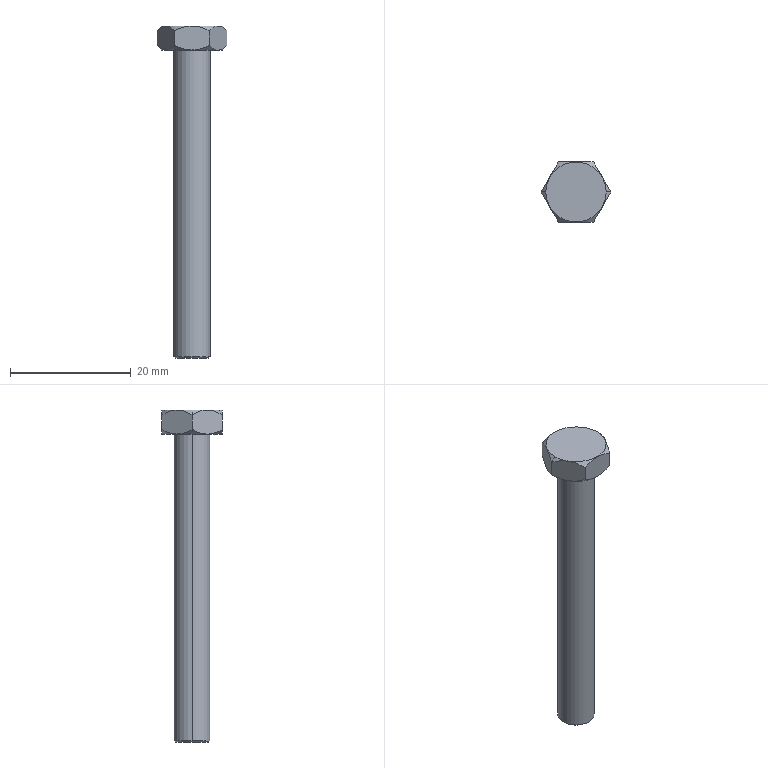Part | STEP file | 1 solid | 17 faces | box 11.547 x 10 x 55 mm | volume 1784 mm3 | plane 9 | cone 6 | cylinder 2 | commonest cylinder face diameters 6 x2